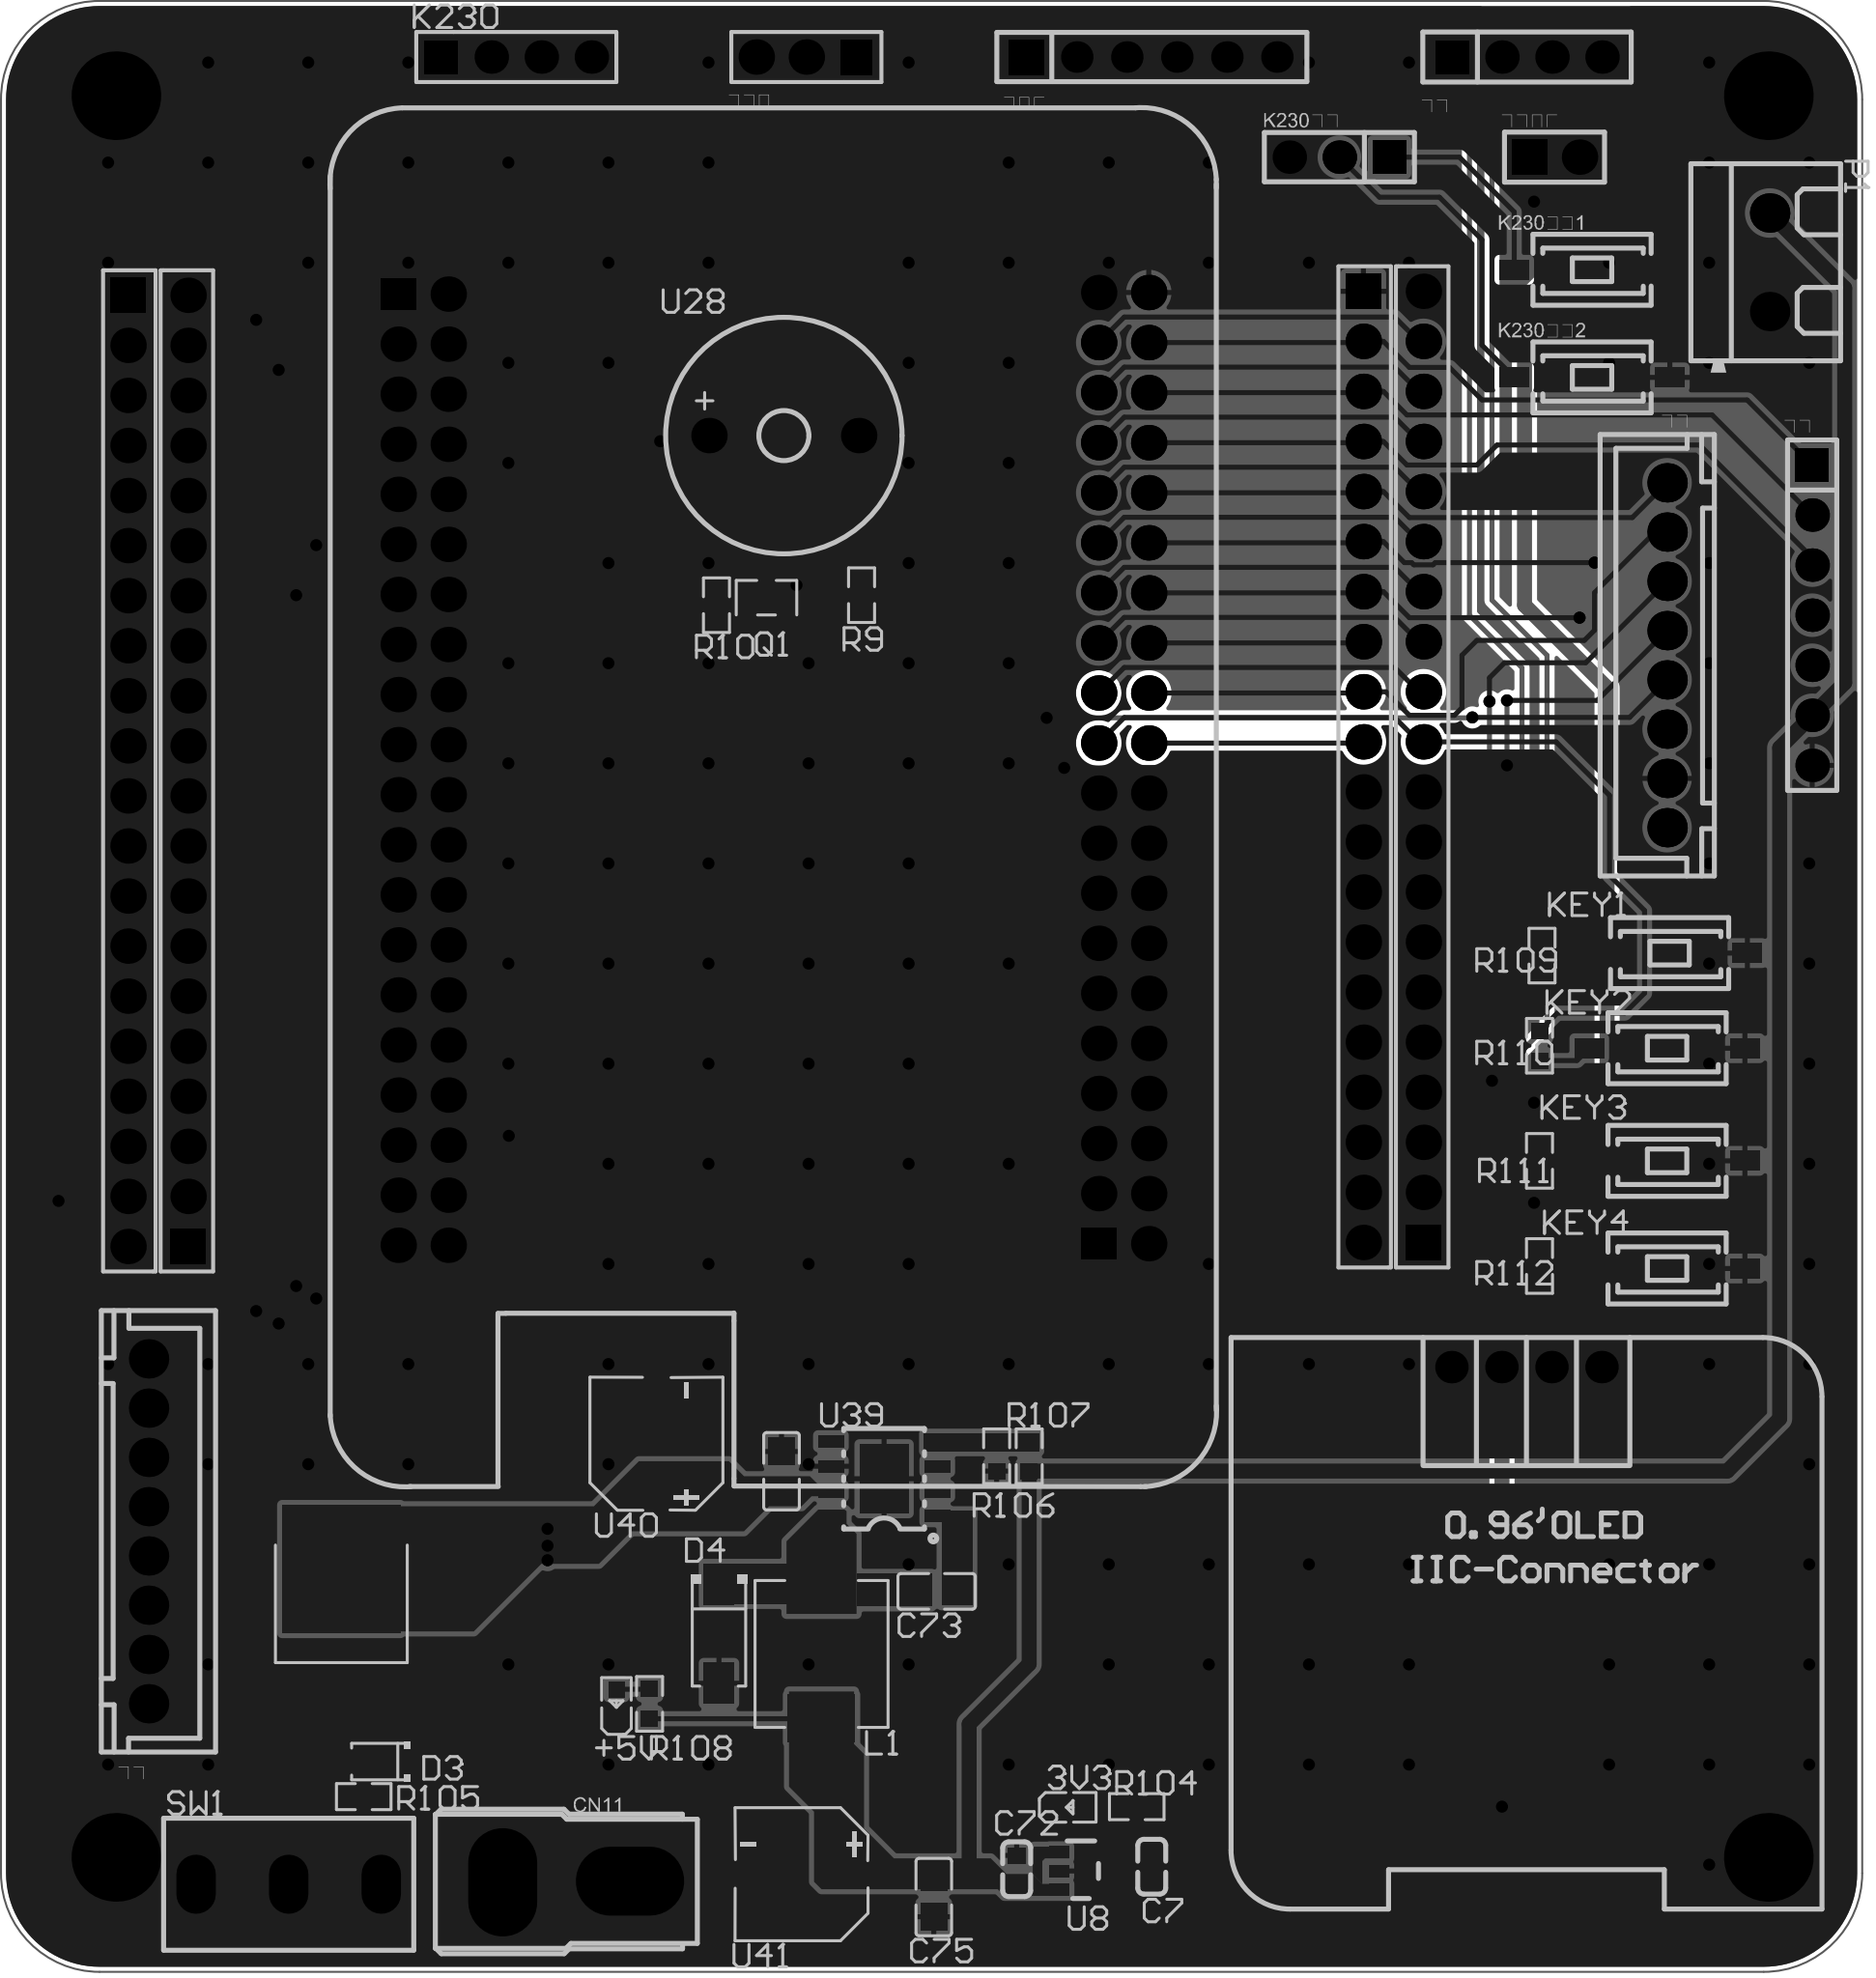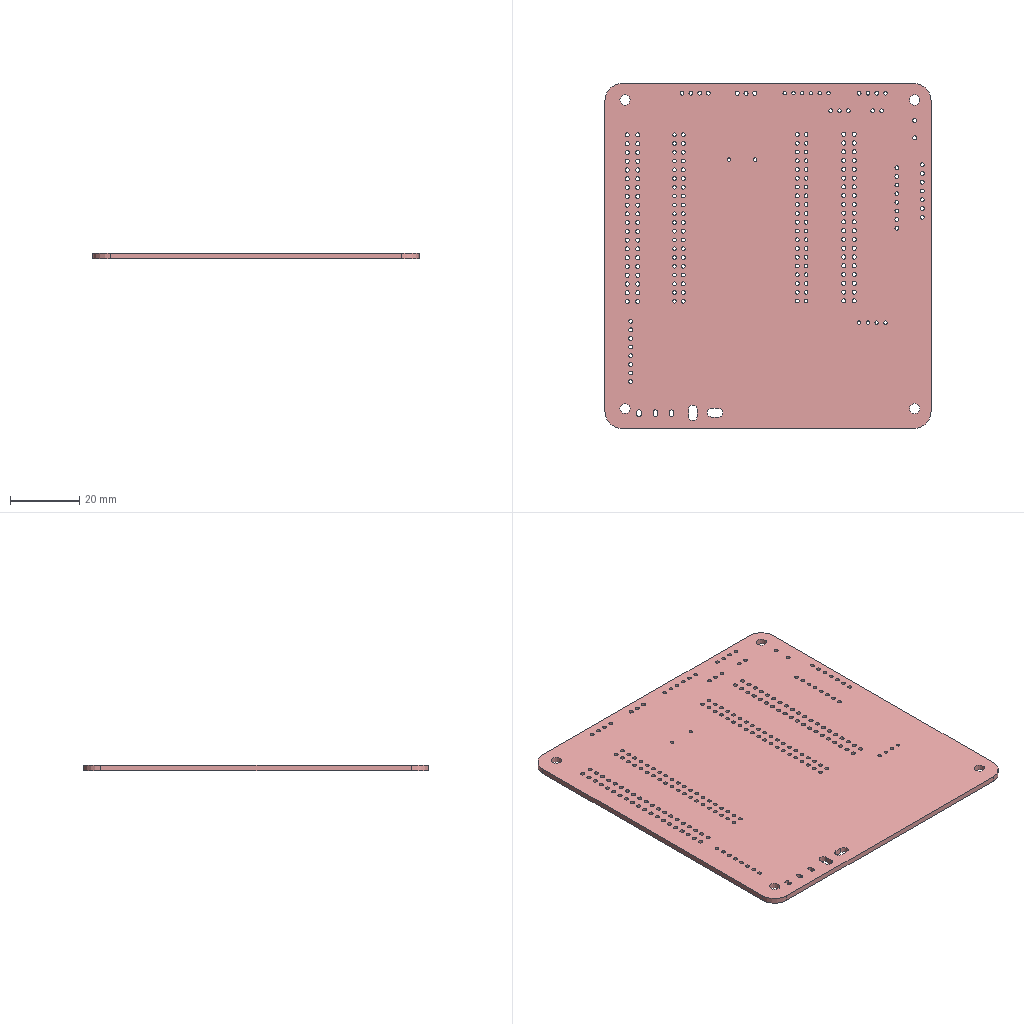Circuit board layout | Altium Designer | box 94.5 x 100 x 1.6 mm
Layer stack:
# Altium Designer layer stack of  (unit mm; dielectric type: 0 none, 1 core, 2 prepreg, 3 surface material)
index,name,kind,layer,copper_thickness_mm,dielectric_type,dielectric_thickness_mm,dielectric_material,dielectric_constant
0,Top Paste Mask Layer,other,,,,,,
1,Top Silkscreen Layer,other,,,,,,
2,Top Solder Mask Layer,dielectric,,,3,0.01,,3.3
3,Top Layer,copper,Top Layer,0.035,,,,
4,Dielectric1,dielectric,,,3,1.51,FR4,4.5
5,Bottom Layer,copper,Bottom Layer,0.035,,,,
6,Bottom Solder Mask Layer,dielectric,,,3,0.01,,3.3
7,Bottom Silkscreen Layer,other,,,,,,
8,Bottom Paste Mask Layer,other,,,,,,
# drill layer pairs: low layer,high layer
drill_pair,Top Layer,Bottom Layer
Part placement:
Designator,Comment,Layer,Footprint,Center-X(mm),Center-Y(mm),Rotation
C7,1uF,TopLayer,C0603,141.351,88.773,90
C72,1uF,TopLayer,C0603,134.493,88.646,270
C73,100nF,TopLayer,C0805,130.429,102.743,180
C74,100nF,TopLayer,C0805,122.555,108.839,270
C75,100nF,TopLayer,C0805,130.286,87.233,90
激光模块,,TopLayer,HDR-TH_2P-P2.54-V-M-1,161.798,175.514,0
CN11,AM-1015B-M,TopLayer,CONN-TH_AM-1015B-M,111.633,88.011,0
D3,BZT52C16,TopLayer,SOD-123_L2.7-W1.6-LS3.7-RD,102.108,94.107,180
D4,SS54,TopLayer,SMA_L4.4-W2.8-LS5.4-R-RD,119.38,100.584,270
H1,,TopLayer,HDR-TH_20P-P2.54-V-M-1,89.383,144.374,270
H2,,TopLayer,HDR-TH_20P-P2.54-V-M-1,92.431,144.374,90
H3,,TopLayer,HDR-TH_20P-P2.54-V-M-1,155.143,144.577,90
H4,,TopLayer,HDR-TH_20P-P2.54-V-M-1,152.095,144.577,270
L1,4.7uH,TopLayer,IND-SMD_L7.3-W6.6,124.587,99.568,90
3V3,,TopLayer,LED_0603,137.135,91.779,0
Q1,S8550,TopLayer,SOT-23-3_L2.9-W1.6-P1.90-LS2.8-BR,121.793,153.162,270
Q2,HY19P03D,TopLayer,TO-252-2_L6.6-W6.1-P4.57-LS9.9-TL-CW,100.203,100.584,90
R9,100Ω,TopLayer,R0603,126.619,153.289,90
R10,100Ω,TopLayer,R0603,119.253,152.781,90
R104,10K,TopLayer,R0603,140.589,91.821,180
R105,10kΩ,TopLayer,R0603,101.346,92.329,180
R106,3.24K,TopLayer,R0603,133.477,109.601,90
R107,10K,TopLayer,R0603,135.128,109.601,270
R108,4.7K,TopLayer,R0603,115.857,97.035,270
U4,,TopLayer,COMM-TH_LCKFB-TMX-MSPM0G3507,122.149,144.475,0
U8,TLV75733PDBVR,TopLayer,SOT-23-5_L2.9-W1.6-P0.95-LS2.8-BL,137.757,88.557,270
K230按键,K230按键,TopLayer,HDR-TH_3P-P2.54-V-M,150.876,175.514,180
P1,KF301-2P接线端子,TopLayer,CONN-TH_XY301V-A-5.0-2P,172.72,170.18,270
R109,100Ω,TopLayer,R0603,161.163,135.001,90
U28,2.6kHz,TopLayer,BUZ-TH_BD12.0-P7.60-D0.6-FD,122.674,161.387,0
R110,100Ω,TopLayer,R0603,161.036,130.429,90
R111,100Ω,TopLayer,R0603,161.036,124.587,90
U39,TPS5430DDAR,TopLayer,ESOP-8_L4.9-W3.9-P1.27-LS6.0-TL-EP,127.762,108.458,180
U40,220uF,TopLayer,CAP-SMD_BD6.3-L6.6-W6.6-LS7.2-FD,116.205,110.236,90
U41,220uF,TopLayer,CAP-SMD_BD6.3-L6.6-W6.6-LS7.2-FD,123.571,88.392,180
SW1,SS-12D10L5,TopLayer,SW-TH_SS-12D10L5,97.536,87.884,180
R112,100Ω,TopLayer,R0603,161.036,119.253,90
+5V,,TopLayer,LED_0603,114.181,96.977,90
驱动板,2.54mm-1*3P 直针,TopLayer,HDR-TH_3P-P2.54-V-M-1,123.817,180.594,180
测距,PM2.54-1*4,TopLayer,HDR-TH_4P-P2.54-V-F,160.401,180.594,0
灰度,PZ2.54-1*7,TopLayer,HDR-TH_7P-P2.54-V-M,174.879,152.273,270
陀螺仪,2.54-1*6P母,TopLayer,HDR-TH_6P-P2.54-V-F,141.356,180.594,0
KEY3,轻触按键3*6*2.5,TopLayer,SW-SMD_L6.0-W3.6-LS8.0,167.513,124.587,0
KEY2,轻触按键3*6*2.5,TopLayer,SW-SMD_L6.0-W3.6-LS8.0,167.513,130.302,0
KEY1,轻触按键3*6*2.5,TopLayer,SW-SMD_L6.0-W3.6-LS8.0,167.64,135.128,0
K230按键1,轻触按键3*6*2.5,TopLayer,SW-SMD_L6.0-W3.6-LS8.0,163.703,169.799,0
K230按键2,轻触按键3*6*2.5,TopLayer,SW-SMD_L6.0-W3.6-LS8.0,163.703,164.338,0
KEY4,轻触按键3*6*2.5,TopLayer,SW-SMD_L6.0-W3.6-LS8.0,167.513,119.126,0
U5,,TopLayer,0.96OLED_4P,160.375,114.123,0
水平,水平,TopLayer,CONN-TH_8P-P2.50-XH2.54-8P,90.424,105.791,90
竖直,竖直,TopLayer,CONN-TH_8P-P2.50-XH2.54-8P,167.513,150.241,270
K230,2.54*4单排,TopLayer,HDR-TH_4P-P2.54-V-M-1,109.093,180.594,0
Pad and via stacks:
# Altium Designer via and pad stacks of  (unit mm). Each distinct definition once, with the count of objects using it.
# via: kind,start_layer,end_layer,hole_mm,diameter_mm,mode(0 simple;1 top-mid-bottom;2 full stack),diameter_per_layer,count,example_net
# pad: kind,layer,hole_mm,hole_type(0 round;1 square;2 slot),plating,top_size,top_shape(1 round;2 rect;3 octagon;9 rounded rect),mid_size,bottom_size,mode,footprint,size_per_layer,count,example
pad,Multi-Layer,3,0,plated,4.501x4.501,1,4.501x4.501,4.501x4.501,0,,,4,1
pad,Multi-Layer,1.1,0,plated,1.8x1.8,1,1.8x1.8,1.8x1.8,0,HDR-TH_2P-P2.54-V-M-1,,1,\u6FC0\u5149\u6A21\u5757.2
pad,Multi-Layer,1.1,0,plated,1.8x1.8,2,1.8x1.8,1.8x1.8,0,HDR-TH_2P-P2.54-V-M-1,,1,\u6FC0\u5149\u6A21\u5757.1
pad,Multi-Layer,2.5,2,plated,3.5x5.5,1,3.5x5.5,3.5x5.5,0,CONN-TH_AM-1015B-M,,2,CN11.1
pad,Multi-Layer,1.2,0,plated,1.8x1.8,1,1.8x1.8,1.8x1.8,0,HDR-TH_20P-P2.54-V-M-1,,76,H1.20
pad,Multi-Layer,1.2,0,plated,1.8x1.8,2,1.8x1.8,1.8x1.8,0,HDR-TH_20P-P2.54-V-M-1,,4,H1.1
pad,Multi-Layer,1.1,0,plated,1.8x1.8,1,1.8x1.8,1.8x1.8,0,COMM-TH_LCKFB-TMX-MSPM0G3507,,78,U4.80
pad,Multi-Layer,1.1,0,plated,1.575x1.8,2,1.575x1.8,1.575x1.8,0,COMM-TH_LCKFB-TMX-MSPM0G3507,,2,U4.41
pad,Multi-Layer,1.1,0,plated,1.7x1.7,2,1.7x1.7,1.7x1.7,0,HDR-TH_3P-P2.54-V-M,,1,K230\u6309\u952E.1
pad,Multi-Layer,1.1,0,plated,1.7x1.7,1,1.7x1.7,1.7x1.7,0,HDR-TH_3P-P2.54-V-M,,2,K230\u6309\u952E.2
pad,Multi-Layer,1.2,0,plated,2x2,1,2x2,2x2,0,CONN-TH_XY301V-A-5.0-2P,,2,P1.1
pad,Multi-Layer,1,0,plated,1.8x1.8,1,1.8x1.8,1.8x1.8,0,BUZ-TH_BD12.0-P7.60-D0.6-FD,,2,U28.2
pad,Multi-Layer,1.3,2,plated,2x3,1,2x3,2x3,0,SW-TH_SS-12D10L5,,3,SW1.1
pad,Multi-Layer,1.2,0,plated,1.8x1.8,1,1.8x1.8,1.8x1.8,0,HDR-TH_3P-P2.54-V-M-1,,2,\u9A71\u52A8\u677F.3
pad,Multi-Layer,1.2,0,plated,1.575x1.8,2,1.575x1.8,1.575x1.8,0,HDR-TH_3P-P2.54-V-M-1,,1,\u9A71\u52A8\u677F.1
pad,Multi-Layer,1.1,0,plated,1.7x1.7,2,1.7x1.7,1.7x1.7,0,HDR-TH_4P-P2.54-V-F,,1,\u6D4B\u8DDD.1
pad,Multi-Layer,1.1,0,plated,1.7x1.7,1,1.7x1.7,1.7x1.7,0,HDR-TH_4P-P2.54-V-F,,3,\u6D4B\u8DDD.2
pad,Multi-Layer,1.1,0,plated,1.7x1.7,2,1.7x1.7,1.7x1.7,0,HDR-TH_7P-P2.54-V-M,,1,\u7070\u5EA6.1
pad,Multi-Layer,1.1,0,plated,1.7x1.7,1,1.7x1.7,1.7x1.7,0,HDR-TH_7P-P2.54-V-M,,6,\u7070\u5EA6.2
pad,Multi-Layer,1.02,0,plated,1.6x1.6,1,1.6x1.6,1.6x1.6,0,HDR-TH_6P-P2.54-V-F,,5,\u9640\u87BA\u4EEA.6
pad,Multi-Layer,1.02,0,plated,1.8x1.8,2,1.8x1.8,1.8x1.8,0,HDR-TH_6P-P2.54-V-F,,1,\u9640\u87BA\u4EEA.1
pad,Multi-Layer,1,0,plated,1.65x1.65,1,1.65x1.65,1.65x1.65,0,0.96OLED_4P,,4,U5.4
pad,Multi-Layer,1.1,0,plated,2x2,1,2x2,2x2,0,CONN-TH_8P-P2.50-XH2.54-8P,,16,\u6C34\u5E73.1
pad,Multi-Layer,1.1,0,plated,1.7x1.7,2,1.7x1.7,1.7x1.7,0,HDR-TH_4P-P2.54-V-M-1,,1,K230.1
pad,Multi-Layer,1.1,0,plated,1.7x1.7,1,1.7x1.7,1.7x1.7,0,HDR-TH_4P-P2.54-V-M-1,,3,K230.2
pad,Top Layer,0,0,plated,0.8x0.9,2,0.8x0.9,0.8x0.9,0,C0603,,4,C7.2
pad,Top Layer,0,0,plated,1.41x1.35,2,1.41x1.35,1.41x1.35,0,C0805,,6,C73.2
pad,Top Layer,0,0,plated,0.91x1.22,2,0.91x1.22,0.91x1.22,0,SOD-123_L2.7-W1.6-LS3.7-RD,,2,D3.2
pad,Top Layer,0,0,plated,2.062x1.539,2,2.062x1.539,2.062x1.539,0,SMA_L4.4-W2.8-LS5.4-R-RD,,2,D4.1
pad,Top Layer,0,0,plated,2.424x3.42,2,2.424x3.42,2.424x3.42,0,IND-SMD_L7.3-W6.6,,2,L1.1
pad,Top Layer,0,0,plated,0.8001x0.8001,2,0.8001x0.8001,0.8001x0.8001,0,LED_0603,,4,3V3.1
pad,Top Layer,0,0,plated,1.07x0.6,2,1.07x0.6,1.07x0.6,0,SOT-23-3_L2.9-W1.6-P1.90-LS2.8-BR,,3,Q1.1
pad,Top Layer,0,0,plated,6.5x6,2,6.5x6,6.5x6,0,TO-252-2_L6.6-W6.1-P4.57-LS9.9-TL-CW,,1,Q2.2
pad,Top Layer,0,0,plated,2.8x1.3,2,2.8x1.3,2.8x1.3,0,TO-252-2_L6.6-W6.1-P4.57-LS9.9-TL-CW,,2,Q2.1
pad,Top Layer,0,0,plated,0.8065x0.864,2,0.8065x0.864,0.8065x0.864,0,R0603,,22,R9.2
pad,Top Layer,0,0,plated,0.6x1,2,0.6x1,0.6x1,0,SOT-23-5_L2.9-W1.6-P0.95-LS2.8-BL,,5,U8.5
pad,Top Layer,0,0,plated,1.3x0.6,2,1.3x0.6,1.3x0.6,0,ESOP-8_L4.9-W3.9-P1.27-LS6.0-TL-EP,,8,U39.1
pad,Top Layer,0,0,plated,2.5x3.5,2,2.5x3.5,2.5x3.5,0,ESOP-8_L4.9-W3.9-P1.27-LS6.0-TL-EP,,1,U39.9
pad,Top Layer,0,0,plated,3.5x1.2,2,3.5x1.2,3.5x1.2,0,CAP-SMD_BD6.3-L6.6-W6.6-LS7.2-FD,,4,U40.2
pad,Top Layer,0,0,plated,1.5x1,2,1.5x1,1.5x1,0,SW-SMD_L6.0-W3.6-LS8.0,,12,KEY3.1
via,Top Layer,Bottom Layer,0.3048,0.61,0,,182,PA15
Copper pours:
name,layer,net,type(0 solid;1 hatched;2 none)
Bottom Layer-GND,Bottom Layer,GND,0
Top Layer-GND,Top Layer,GND,0